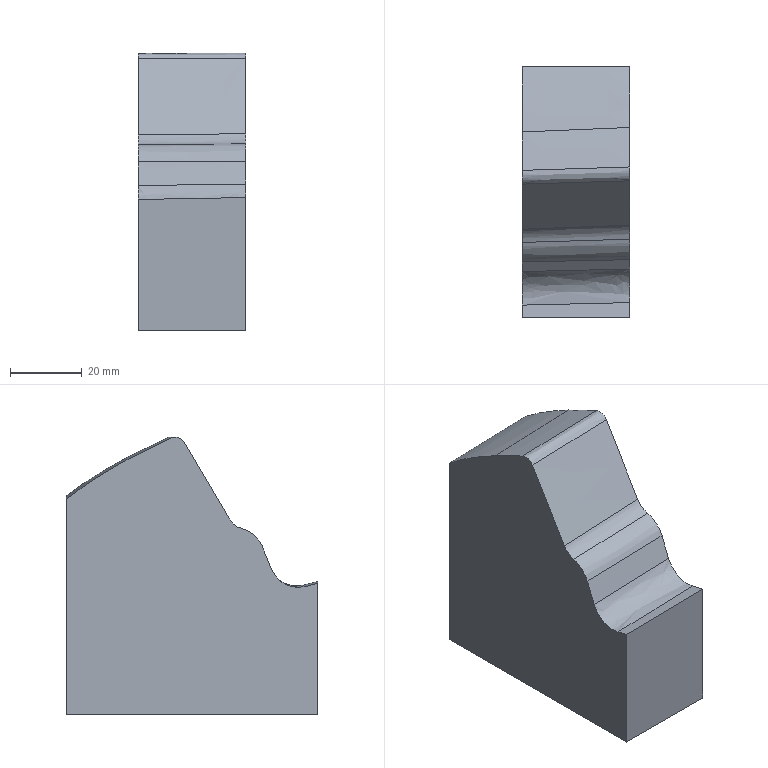Part | NX | features solid 2 | 1 solid | 14 faces | box 30 x 70 x 77.441 mm | volume 125300 mm3 | spline 9 | plane 5
STEP:
#1=CARTESIAN_POINT('',(275.839,786.479,-120.));
#2=VERTEX_POINT('',#1);
#3=CARTESIAN_POINT('',(245.839,786.479,-120.));
#4=VERTEX_POINT('',#3);
#5=CARTESIAN_POINT('',(275.839,786.479,-120.));
#6=DIRECTION('',(1.,0.,0.));
#7=VECTOR('',#6,1000.);
#8=LINE('',#5,#7);
#9=EDGE_CURVE('',#2,#4,#8,.F.);
#10=ORIENTED_EDGE('',*,*,#9,.F.);
#11=CARTESIAN_POINT('',(275.839,716.479,-120.));
#12=VERTEX_POINT('',#11);
#13=CARTESIAN_POINT('',(275.839,776.479,-120.));
#14=DIRECTION('',(0.,-1.,0.));
#15=VECTOR('',#14,1000.);
#16=LINE('',#13,#15);
#17=EDGE_CURVE('',#12,#2,#16,.F.);
#18=ORIENTED_EDGE('',*,*,#17,.F.);
#19=CARTESIAN_POINT('',(245.839,716.479,-120.));
#20=VERTEX_POINT('',#19);
#21=CARTESIAN_POINT('',(275.839,716.479,-120.));
#22=DIRECTION('',(1.,0.,0.));
#23=VECTOR('',#22,1000.);
#24=LINE('',#21,#23);
#25=EDGE_CURVE('',#12,#20,#24,.F.);
#26=ORIENTED_EDGE('',*,*,#25,.T.);
#27=CARTESIAN_POINT('',(245.839,776.479,-120.));
#28=DIRECTION('',(0.,-1.,0.));
#29=VECTOR('',#28,1000.);
#30=LINE('',#27,#29);
#31=EDGE_CURVE('',#20,#4,#30,.F.);
#32=ORIENTED_EDGE('',*,*,#31,.T.);
#33=EDGE_LOOP('',(#10,#18,#26,#32));
#34=FACE_BOUND('',#33,.T.);
#35=CARTESIAN_POINT('',(275.839,776.479,-120.));
#36=DIRECTION('',(0.,0.,1.));
#37=DIRECTION('',(0.,-1.,0.));
#38=AXIS2_PLACEMENT_3D('',#35,#36,#37);
#39=PLANE('',#38);
#40=ADVANCED_FACE('',(#34),#39,.F.);
#41=CARTESIAN_POINT('',(245.839,786.479,-59.905));
#42=VERTEX_POINT('',#41);
#43=CARTESIAN_POINT('',(245.839,768.143,-48.166));
#44=VERTEX_POINT('',#43);
#45=CARTESIAN_POINT('',(245.839,786.479,-59.905));
#46=CARTESIAN_POINT('',(245.839,780.808,-55.303));
#47=CARTESIAN_POINT('',(245.839,774.58,-51.571));
#48=CARTESIAN_POINT('',(245.839,768.143,-48.166));
#49=B_SPLINE_CURVE_WITH_KNOTS('',3,(#45,#46,#47,#48),.UNSPECIFIED.,.F.,.F.,(4,4),(0.,0.02177),.UNSPECIFIED.);
#50=EDGE_CURVE('',#42,#44,#49,.T.);
#51=ORIENTED_EDGE('',*,*,#50,.F.);
#52=CARTESIAN_POINT('',(245.839,786.479,-60.));
#53=DIRECTION('',(0.,0.,-1.));
#54=VECTOR('',#53,1000.);
#55=LINE('',#52,#54);
#56=EDGE_CURVE('',#42,#4,#55,.T.);
#57=ORIENTED_EDGE('',*,*,#56,.T.);
#58=ORIENTED_EDGE('',*,*,#31,.F.);
#59=CARTESIAN_POINT('',(245.839,716.479,-83.363));
#60=VERTEX_POINT('',#59);
#61=CARTESIAN_POINT('',(245.839,716.479,-60.));
#62=DIRECTION('',(0.,0.,-1.));
#63=VECTOR('',#62,1000.);
#64=LINE('',#61,#63);
#65=EDGE_CURVE('',#60,#20,#64,.T.);
#66=ORIENTED_EDGE('',*,*,#65,.F.);
#67=CARTESIAN_POINT('',(245.839,719.964,-84.227));
#68=VERTEX_POINT('',#67);
#69=CARTESIAN_POINT('',(245.839,716.479,-83.363));
#70=CARTESIAN_POINT('',(245.839,717.64,-83.65));
#71=CARTESIAN_POINT('',(245.839,718.801,-83.938));
#72=CARTESIAN_POINT('',(245.839,719.962,-84.226));
#73=B_SPLINE_CURVE_WITH_KNOTS('',3,(#69,#70,#71,#72),.UNSPECIFIED.,.F.,.F.,(4,4),(0.,0.003589),.UNSPECIFIED.);
#74=EDGE_CURVE('',#60,#68,#73,.T.);
#75=ORIENTED_EDGE('',*,*,#74,.T.);
#76=CARTESIAN_POINT('',(245.839,729.312,-79.471));
#77=VERTEX_POINT('',#76);
#78=CARTESIAN_POINT('',(245.839,719.965,-84.227));
#79=CARTESIAN_POINT('',(245.839,721.832,-84.691));
#80=CARTESIAN_POINT('',(245.839,725.84,-84.214));
#81=CARTESIAN_POINT('',(245.839,728.588,-81.253));
#82=CARTESIAN_POINT('',(245.839,729.312,-79.471));
#83=B_SPLINE_CURVE_WITH_KNOTS('',3,(#78,#79,#80,#81,#82),.UNSPECIFIED.,.F.,.F.,(4,1,4),(0.,0.005687,0.01137),.UNSPECIFIED.);
#84=EDGE_CURVE('',#68,#77,#83,.T.);
#85=ORIENTED_EDGE('',*,*,#84,.T.);
#86=CARTESIAN_POINT('',(245.839,731.981,-72.901));
#87=VERTEX_POINT('',#86);
#88=CARTESIAN_POINT('',(245.839,729.312,-79.472));
#89=CARTESIAN_POINT('',(245.839,730.201,-77.282));
#90=CARTESIAN_POINT('',(245.839,731.091,-75.092));
#91=CARTESIAN_POINT('',(245.839,731.98,-72.902));
#92=B_SPLINE_CURVE_WITH_KNOTS('',3,(#88,#89,#90,#91),.UNSPECIFIED.,.F.,.F.,(4,4),(0.00003288,0.007123),.UNSPECIFIED.);
#93=EDGE_CURVE('',#77,#87,#92,.T.);
#94=ORIENTED_EDGE('',*,*,#93,.T.);
#95=CARTESIAN_POINT('',(245.839,737.4,-68.162));
#96=VERTEX_POINT('',#95);
#97=CARTESIAN_POINT('',(245.839,731.981,-72.9));
#98=CARTESIAN_POINT('',(245.839,732.926,-70.575));
#99=CARTESIAN_POINT('',(245.839,734.971,-68.787));
#100=CARTESIAN_POINT('',(245.839,737.401,-68.162));
#101=B_SPLINE_CURVE_WITH_KNOTS('',3,(#97,#98,#99,#100),.UNSPECIFIED.,.F.,.F.,(4,4),(0.,0.007469),.UNSPECIFIED.);
#102=EDGE_CURVE('',#87,#96,#101,.T.);
#103=ORIENTED_EDGE('',*,*,#102,.T.);
#104=CARTESIAN_POINT('',(245.839,741.078,-65.393));
#105=VERTEX_POINT('',#104);
#106=CARTESIAN_POINT('',(245.839,737.4,-68.162));
#107=CARTESIAN_POINT('',(245.839,738.935,-67.766));
#108=CARTESIAN_POINT('',(245.839,740.274,-66.759));
#109=CARTESIAN_POINT('',(245.839,741.078,-65.393));
#110=B_SPLINE_CURVE_WITH_KNOTS('',3,(#106,#107,#108,#109),.UNSPECIFIED.,.F.,.F.,(4,4),(0.,0.004726),.UNSPECIFIED.);
#111=EDGE_CURVE('',#96,#105,#110,.T.);
#112=ORIENTED_EDGE('',*,*,#111,.T.);
#113=CARTESIAN_POINT('',(245.839,753.598,-44.132));
#114=VERTEX_POINT('',#113);
#115=CARTESIAN_POINT('',(245.839,741.078,-65.394));
#116=CARTESIAN_POINT('',(245.839,745.251,-58.307));
#117=CARTESIAN_POINT('',(245.839,749.425,-51.219));
#118=CARTESIAN_POINT('',(245.839,753.598,-44.132));
#119=B_SPLINE_CURVE_WITH_KNOTS('',3,(#115,#116,#117,#118),.UNSPECIFIED.,.F.,.F.,(4,4),(0.000195,0.02487),.UNSPECIFIED.);
#120=EDGE_CURVE('',#105,#114,#119,.T.);
#121=ORIENTED_EDGE('',*,*,#120,.T.);
#122=CARTESIAN_POINT('',(245.839,757.433,-42.927));
#123=VERTEX_POINT('',#122);
#124=CARTESIAN_POINT('',(245.839,753.598,-44.132));
#125=CARTESIAN_POINT('',(245.839,753.974,-43.495));
#126=CARTESIAN_POINT('',(245.839,755.203,-42.538));
#127=CARTESIAN_POINT('',(245.839,756.759,-42.623));
#128=CARTESIAN_POINT('',(245.839,757.433,-42.927));
#129=B_SPLINE_CURVE_WITH_KNOTS('',3,(#124,#125,#126,#127,#128),.UNSPECIFIED.,.F.,.F.,(4,1,4),(0.,0.002188,0.004376),.UNSPECIFIED.);
#130=EDGE_CURVE('',#114,#123,#129,.T.);
#131=ORIENTED_EDGE('',*,*,#130,.T.);
#132=CARTESIAN_POINT('',(245.839,768.143,-48.166));
#133=CARTESIAN_POINT('',(245.839,764.629,-46.307));
#134=CARTESIAN_POINT('',(245.839,761.057,-44.561));
#135=CARTESIAN_POINT('',(245.839,757.433,-42.927));
#136=B_SPLINE_CURVE_WITH_KNOTS('',3,(#132,#133,#134,#135),.UNSPECIFIED.,.F.,.F.,(4,4),(0.002124,0.01405),.UNSPECIFIED.);
#137=EDGE_CURVE('',#44,#123,#136,.T.);
#138=ORIENTED_EDGE('',*,*,#137,.F.);
#139=EDGE_LOOP('',(#51,#57,#58,#66,#75,#85,#94,#103,#112,#121,#131,#138));
#140=FACE_BOUND('',#139,.T.);
#141=CARTESIAN_POINT('',(245.839,726.479,-60.));
#142=DIRECTION('',(-1.,0.,0.));
#143=DIRECTION('',(0.,-1.,0.));
#144=AXIS2_PLACEMENT_3D('',#141,#142,#143);
#145=PLANE('',#144);
#146=ADVANCED_FACE('',(#140),#145,.T.);
#147=CARTESIAN_POINT('',(275.839,716.479,-82.838));
#148=VERTEX_POINT('',#147);
#149=CARTESIAN_POINT('',(275.839,716.479,-60.));
#150=DIRECTION('',(0.,0.,-1.));
#151=VECTOR('',#150,1000.);
#152=LINE('',#149,#151);
#153=EDGE_CURVE('',#148,#12,#152,.T.);
#154=ORIENTED_EDGE('',*,*,#153,.F.);
#155=CARTESIAN_POINT('',(275.839,716.479,-82.838));
#156=CARTESIAN_POINT('',(265.839,716.479,-83.013));
#157=CARTESIAN_POINT('',(255.839,716.479,-83.188));
#158=CARTESIAN_POINT('',(245.839,716.479,-83.363));
#159=B_SPLINE_CURVE_WITH_KNOTS('',3,(#155,#156,#157,#158),.UNSPECIFIED.,.F.,.F.,(4,4),(0.,0.03),.UNSPECIFIED.);
#160=EDGE_CURVE('',#148,#60,#159,.T.);
#161=ORIENTED_EDGE('',*,*,#160,.T.);
#162=ORIENTED_EDGE('',*,*,#65,.T.);
#163=ORIENTED_EDGE('',*,*,#25,.F.);
#164=EDGE_LOOP('',(#154,#161,#162,#163));
#165=FACE_BOUND('',#164,.T.);
#166=CARTESIAN_POINT('',(275.839,716.479,-60.));
#167=DIRECTION('',(0.,-1.,0.));
#168=DIRECTION('',(1.,0.,0.));
#169=AXIS2_PLACEMENT_3D('',#166,#167,#168);
#170=PLANE('',#169);
#171=ADVANCED_FACE('',(#165),#170,.T.);
#172=CARTESIAN_POINT('',(275.839,786.479,-58.959));
#173=VERTEX_POINT('',#172);
#174=CARTESIAN_POINT('',(275.839,786.479,-60.));
#175=DIRECTION('',(0.,0.,-1.));
#176=VECTOR('',#175,1000.);
#177=LINE('',#174,#176);
#178=EDGE_CURVE('',#173,#2,#177,.T.);
#179=ORIENTED_EDGE('',*,*,#178,.F.);
#180=CARTESIAN_POINT('',(275.839,769.372,-48.194));
#181=VERTEX_POINT('',#180);
#182=CARTESIAN_POINT('',(275.839,786.479,-58.959));
#183=CARTESIAN_POINT('',(275.839,781.136,-54.8));
#184=CARTESIAN_POINT('',(275.839,775.346,-51.354));
#185=CARTESIAN_POINT('',(275.839,769.374,-48.195));
#186=B_SPLINE_CURVE_WITH_KNOTS('',3,(#182,#183,#184,#185),.UNSPECIFIED.,.F.,.F.,(4,4),(0.,0.02021),.UNSPECIFIED.);
#187=EDGE_CURVE('',#173,#181,#186,.T.);
#188=ORIENTED_EDGE('',*,*,#187,.T.);
#189=CARTESIAN_POINT('',(275.839,758.369,-42.827));
#190=VERTEX_POINT('',#189);
#191=CARTESIAN_POINT('',(275.839,769.371,-48.193));
#192=CARTESIAN_POINT('',(275.839,765.763,-46.285));
#193=CARTESIAN_POINT('',(275.839,762.092,-44.496));
#194=CARTESIAN_POINT('',(275.839,758.368,-42.826));
#195=B_SPLINE_CURVE_WITH_KNOTS('',3,(#191,#192,#193,#194),.UNSPECIFIED.,.F.,.F.,(4,4),(0.001603,0.01385),.UNSPECIFIED.);
#196=EDGE_CURVE('',#181,#190,#195,.T.);
#197=ORIENTED_EDGE('',*,*,#196,.T.);
#198=CARTESIAN_POINT('',(275.839,754.512,-44.025));
#199=VERTEX_POINT('',#198);
#200=CARTESIAN_POINT('',(275.839,754.512,-44.025));
#201=CARTESIAN_POINT('',(275.839,755.263,-42.743));
#202=CARTESIAN_POINT('',(275.839,757.014,-42.219));
#203=CARTESIAN_POINT('',(275.839,758.37,-42.827));
#204=B_SPLINE_CURVE_WITH_KNOTS('',3,(#200,#201,#202,#203),.UNSPECIFIED.,.F.,.F.,(4,4),(0.,0.004395),.UNSPECIFIED.);
#205=EDGE_CURVE('',#199,#190,#204,.T.);
#206=ORIENTED_EDGE('',*,*,#205,.F.);
#207=CARTESIAN_POINT('',(275.839,742.202,-65.047));
#208=VERTEX_POINT('',#207);
#209=CARTESIAN_POINT('',(275.839,742.203,-65.046));
#210=CARTESIAN_POINT('',(275.839,746.307,-58.039));
#211=CARTESIAN_POINT('',(275.839,750.41,-51.032));
#212=CARTESIAN_POINT('',(275.839,754.512,-44.025));
#213=B_SPLINE_CURVE_WITH_KNOTS('',3,(#209,#210,#211,#212),.UNSPECIFIED.,.F.,.F.,(4,4),(0.0005091,0.02487),.UNSPECIFIED.);
#214=EDGE_CURVE('',#208,#199,#213,.T.);
#215=ORIENTED_EDGE('',*,*,#214,.F.);
#216=CARTESIAN_POINT('',(275.839,738.294,-67.882));
#217=VERTEX_POINT('',#216);
#218=CARTESIAN_POINT('',(275.839,738.307,-67.879));
#219=CARTESIAN_POINT('',(275.839,739.931,-67.523));
#220=CARTESIAN_POINT('',(275.839,741.362,-66.483));
#221=CARTESIAN_POINT('',(275.839,742.202,-65.048));
#222=B_SPLINE_CURVE_WITH_KNOTS('',3,(#218,#219,#220,#221),.UNSPECIFIED.,.F.,.F.,(4,4),(0.,0.004958),.UNSPECIFIED.);
#223=EDGE_CURVE('',#217,#208,#222,.T.);
#224=ORIENTED_EDGE('',*,*,#223,.F.);
#225=CARTESIAN_POINT('',(275.839,732.598,-72.709));
#226=VERTEX_POINT('',#225);
#227=CARTESIAN_POINT('',(275.839,732.601,-72.701));
#228=CARTESIAN_POINT('',(275.839,733.576,-70.285));
#229=CARTESIAN_POINT('',(275.839,735.748,-68.447));
#230=CARTESIAN_POINT('',(275.839,738.29,-67.883));
#231=B_SPLINE_CURVE_WITH_KNOTS('',3,(#227,#228,#229,#230),.UNSPECIFIED.,.F.,.F.,(4,4),(0.,0.007755),.UNSPECIFIED.);
#232=EDGE_CURVE('',#226,#217,#231,.T.);
#233=ORIENTED_EDGE('',*,*,#232,.F.);
#234=CARTESIAN_POINT('',(275.839,730.018,-79.103));
#235=VERTEX_POINT('',#234);
#236=CARTESIAN_POINT('',(275.839,730.018,-79.103));
#237=CARTESIAN_POINT('',(275.839,730.878,-76.973));
#238=CARTESIAN_POINT('',(275.839,731.737,-74.842));
#239=CARTESIAN_POINT('',(275.839,732.597,-72.712));
#240=B_SPLINE_CURVE_WITH_KNOTS('',3,(#236,#237,#238,#239),.UNSPECIFIED.,.F.,.F.,(4,4),(0.00002376,0.006916),.UNSPECIFIED.);
#241=EDGE_CURVE('',#235,#226,#240,.T.);
#242=ORIENTED_EDGE('',*,*,#241,.F.);
#243=CARTESIAN_POINT('',(275.839,720.661,-83.875));
#244=VERTEX_POINT('',#243);
#245=CARTESIAN_POINT('',(275.839,720.665,-83.876));
#246=CARTESIAN_POINT('',(275.839,722.534,-84.341));
#247=CARTESIAN_POINT('',(275.839,726.55,-83.861));
#248=CARTESIAN_POINT('',(275.839,729.298,-80.89));
#249=CARTESIAN_POINT('',(275.839,730.018,-79.103));
#250=B_SPLINE_CURVE_WITH_KNOTS('',3,(#245,#246,#247,#248,#249),.UNSPECIFIED.,.F.,.F.,(4,1,4),(0.,0.005697,0.01139),.UNSPECIFIED.);
#251=EDGE_CURVE('',#244,#235,#250,.T.);
#252=ORIENTED_EDGE('',*,*,#251,.F.);
#253=CARTESIAN_POINT('',(275.839,716.479,-82.838));
#254=CARTESIAN_POINT('',(275.839,717.873,-83.183));
#255=CARTESIAN_POINT('',(275.839,719.266,-83.528));
#256=CARTESIAN_POINT('',(275.839,720.66,-83.875));
#257=B_SPLINE_CURVE_WITH_KNOTS('',3,(#253,#254,#255,#256),.UNSPECIFIED.,.F.,.F.,(4,4),(0.,0.004308),.UNSPECIFIED.);
#258=EDGE_CURVE('',#148,#244,#257,.T.);
#259=ORIENTED_EDGE('',*,*,#258,.F.);
#260=ORIENTED_EDGE('',*,*,#153,.T.);
#261=ORIENTED_EDGE('',*,*,#17,.T.);
#262=EDGE_LOOP('',(#179,#188,#197,#206,#215,#224,#233,#242,#252,#259,#260,#261));
#263=FACE_BOUND('',#262,.T.);
#264=CARTESIAN_POINT('',(275.839,726.479,-60.));
#265=DIRECTION('',(-1.,0.,0.));
#266=DIRECTION('',(0.,-1.,0.));
#267=AXIS2_PLACEMENT_3D('',#264,#265,#266);
#268=PLANE('',#267);
#269=ADVANCED_FACE('',(#263),#268,.F.);
#270=ORIENTED_EDGE('',*,*,#56,.F.);
#271=CARTESIAN_POINT('',(245.839,786.479,-59.905));
#272=CARTESIAN_POINT('',(255.839,786.479,-59.575));
#273=CARTESIAN_POINT('',(265.839,786.479,-59.26));
#274=CARTESIAN_POINT('',(275.839,786.479,-58.959));
#275=B_SPLINE_CURVE_WITH_KNOTS('',3,(#271,#272,#273,#274),.UNSPECIFIED.,.F.,.F.,(4,4),(0.,0.03001),.UNSPECIFIED.);
#276=EDGE_CURVE('',#42,#173,#275,.T.);
#277=ORIENTED_EDGE('',*,*,#276,.T.);
#278=ORIENTED_EDGE('',*,*,#178,.T.);
#279=ORIENTED_EDGE('',*,*,#9,.T.);
#280=EDGE_LOOP('',(#270,#277,#278,#279));
#281=FACE_BOUND('',#280,.T.);
#282=CARTESIAN_POINT('',(275.839,786.479,-60.));
#283=DIRECTION('',(0.,-1.,0.));
#284=DIRECTION('',(1.,0.,0.));
#285=AXIS2_PLACEMENT_3D('',#282,#283,#284);
#286=PLANE('',#285);
#287=ADVANCED_FACE('',(#281),#286,.F.);
#288=ORIENTED_EDGE('',*,*,#276,.F.);
#289=ORIENTED_EDGE('',*,*,#50,.T.);
#290=CARTESIAN_POINT('',(275.839,769.374,-48.195));
#291=CARTESIAN_POINT('',(265.838,768.982,-48.191));
#292=CARTESIAN_POINT('',(255.838,768.573,-48.182));
#293=CARTESIAN_POINT('',(245.839,768.143,-48.166));
#294=B_SPLINE_CURVE_WITH_KNOTS('',3,(#290,#291,#292,#293),.UNSPECIFIED.,.F.,.F.,(4,4),(0.79,0.9686),.UNSPECIFIED.);
#295=EDGE_CURVE('',#181,#44,#294,.T.);
#296=ORIENTED_EDGE('',*,*,#295,.F.);
#297=ORIENTED_EDGE('',*,*,#187,.F.);
#298=EDGE_LOOP('',(#288,#289,#296,#297));
#299=FACE_BOUND('',#298,.T.);
#300=CARTESIAN_POINT('',(276.02,769.382,-48.195));
#301=CARTESIAN_POINT('',(276.026,773.342,-50.29));
#302=CARTESIAN_POINT('',(276.033,777.232,-52.501));
#303=CARTESIAN_POINT('',(276.043,780.983,-54.841));
#304=CARTESIAN_POINT('',(276.04,784.525,-57.337));
#305=CARTESIAN_POINT('',(276.008,787.811,-60.014));
#306=CARTESIAN_POINT('',(269.947,769.144,-48.193));
#307=CARTESIAN_POINT('',(269.952,773.104,-50.288));
#308=CARTESIAN_POINT('',(269.959,776.994,-52.499));
#309=CARTESIAN_POINT('',(269.967,780.745,-54.839));
#310=CARTESIAN_POINT('',(269.963,784.287,-57.335));
#311=CARTESIAN_POINT('',(269.93,787.573,-60.012));
#312=CARTESIAN_POINT('',(263.875,768.9,-48.189));
#313=CARTESIAN_POINT('',(263.878,772.86,-50.284));
#314=CARTESIAN_POINT('',(263.884,776.751,-52.495));
#315=CARTESIAN_POINT('',(263.891,780.502,-54.835));
#316=CARTESIAN_POINT('',(263.886,784.044,-57.331));
#317=CARTESIAN_POINT('',(263.851,787.33,-60.009));
#318=CARTESIAN_POINT('',(257.802,768.651,-48.183));
#319=CARTESIAN_POINT('',(257.804,772.612,-50.278));
#320=CARTESIAN_POINT('',(257.809,776.502,-52.49));
#321=CARTESIAN_POINT('',(257.815,780.253,-54.829));
#322=CARTESIAN_POINT('',(257.808,783.796,-57.325));
#323=CARTESIAN_POINT('',(257.772,787.082,-60.003));
#324=CARTESIAN_POINT('',(251.73,768.397,-48.176));
#325=CARTESIAN_POINT('',(251.73,772.357,-50.271));
#326=CARTESIAN_POINT('',(251.733,776.248,-52.482));
#327=CARTESIAN_POINT('',(251.738,779.998,-54.821));
#328=CARTESIAN_POINT('',(251.73,783.541,-57.317));
#329=CARTESIAN_POINT('',(251.692,786.827,-59.995));
#330=CARTESIAN_POINT('',(245.658,768.135,-48.166));
#331=CARTESIAN_POINT('',(245.657,772.096,-50.261));
#332=CARTESIAN_POINT('',(245.658,775.987,-52.472));
#333=CARTESIAN_POINT('',(245.661,779.738,-54.811));
#334=CARTESIAN_POINT('',(245.651,783.281,-57.307));
#335=CARTESIAN_POINT('',(245.611,786.567,-59.985));
#336=B_SPLINE_SURFACE_WITH_KNOTS('',5,5,((#300,#301,#302,#303,#304,#305),(#306,#307,#308,#309,#310,#311),(#312,#313,#314,#315,#316,#317),(#318,#319,#320,#321,#322,#323),(#324,#325,#326,#327,#328,#329),(#330,#331,#332,#333,#334,#335)),.UNSPECIFIED.,.F.,.F.,.F.,(6,6),(6,6),(0.8526,0.9789),(0.,0.2902),.PIECEWISE_BEZIER_KNOTS.);
#337=ADVANCED_FACE('',(#299),#336,.F.);
#338=ORIENTED_EDGE('',*,*,#295,.T.);
#339=ORIENTED_EDGE('',*,*,#137,.T.);
#340=CARTESIAN_POINT('',(275.839,758.368,-42.826));
#341=CARTESIAN_POINT('',(265.09,758.062,-42.872));
#342=CARTESIAN_POINT('',(255.09,757.75,-42.906));
#343=CARTESIAN_POINT('',(245.839,757.433,-42.927));
#344=B_SPLINE_CURVE_WITH_KNOTS('',3,(#340,#341,#342,#343),.UNSPECIFIED.,.F.,.F.,(4,4),(0.5417,0.9262),.UNSPECIFIED.);
#345=EDGE_CURVE('',#190,#123,#344,.T.);
#346=ORIENTED_EDGE('',*,*,#345,.F.);
#347=ORIENTED_EDGE('',*,*,#196,.F.);
#348=EDGE_LOOP('',(#338,#339,#346,#347));
#349=FACE_BOUND('',#348,.T.);
#350=CARTESIAN_POINT('',(276.079,757.983,-42.65));
#351=CARTESIAN_POINT('',(276.044,763.838,-45.259));
#352=CARTESIAN_POINT('',(276.019,769.442,-48.227));
#353=CARTESIAN_POINT('',(269.994,757.86,-42.698));
#354=CARTESIAN_POINT('',(269.962,763.701,-45.307));
#355=CARTESIAN_POINT('',(269.941,769.292,-48.272));
#356=CARTESIAN_POINT('',(263.909,757.736,-42.747));
#357=CARTESIAN_POINT('',(263.881,763.564,-45.355));
#358=CARTESIAN_POINT('',(263.863,769.141,-48.317));
#359=CARTESIAN_POINT('',(257.825,757.612,-42.797));
#360=CARTESIAN_POINT('',(257.8,763.425,-45.404));
#361=CARTESIAN_POINT('',(257.786,768.989,-48.362));
#362=CARTESIAN_POINT('',(251.742,757.487,-42.847));
#363=CARTESIAN_POINT('',(251.721,763.285,-45.453));
#364=CARTESIAN_POINT('',(251.71,768.835,-48.408));
#365=CARTESIAN_POINT('',(245.659,757.36,-42.898));
#366=CARTESIAN_POINT('',(245.641,763.144,-45.503));
#367=CARTESIAN_POINT('',(245.634,768.679,-48.455));
#368=B_SPLINE_SURFACE_WITH_KNOTS('',5,2,((#350,#351,#352),(#353,#354,#355),(#356,#357,#358),(#359,#360,#361),(#362,#363,#364),(#365,#366,#367)),.UNSPECIFIED.,.F.,.F.,.F.,(6,6),(3,3),(0.7902,0.97),(0.006349,0.8931),.PIECEWISE_BEZIER_KNOTS.);
#369=ADVANCED_FACE('',(#349),#368,.F.);
#370=ORIENTED_EDGE('',*,*,#205,.T.);
#371=ORIENTED_EDGE('',*,*,#345,.T.);
#372=ORIENTED_EDGE('',*,*,#130,.F.);
#373=CARTESIAN_POINT('',(275.839,754.512,-44.025));
#374=CARTESIAN_POINT('',(265.837,754.225,-44.064));
#375=CARTESIAN_POINT('',(255.837,753.92,-44.099));
#376=CARTESIAN_POINT('',(245.839,753.598,-44.132));
#377=B_SPLINE_CURVE_WITH_KNOTS('',3,(#373,#374,#375,#376),.UNSPECIFIED.,.F.,.F.,(4,4),(0.79,0.969),.UNSPECIFIED.);
#378=EDGE_CURVE('',#114,#199,#377,.F.);
#379=ORIENTED_EDGE('',*,*,#378,.T.);
#380=EDGE_LOOP('',(#370,#371,#372,#379));
#381=FACE_BOUND('',#380,.T.);
#382=CARTESIAN_POINT('',(276.025,758.375,-42.826));
#383=CARTESIAN_POINT('',(276.015,756.977,-42.2));
#384=CARTESIAN_POINT('',(276.012,755.291,-42.703));
#385=CARTESIAN_POINT('',(276.078,754.519,-44.024));
#386=CARTESIAN_POINT('',(269.94,758.202,-42.852));
#387=CARTESIAN_POINT('',(269.931,756.804,-42.225));
#388=CARTESIAN_POINT('',(269.933,755.118,-42.727));
#389=CARTESIAN_POINT('',(269.993,754.345,-44.048));
#390=CARTESIAN_POINT('',(263.855,758.021,-42.876));
#391=CARTESIAN_POINT('',(263.849,756.624,-42.248));
#392=CARTESIAN_POINT('',(263.855,754.938,-42.75));
#393=CARTESIAN_POINT('',(263.909,754.165,-44.071));
#394=CARTESIAN_POINT('',(257.77,757.832,-42.897));
#395=CARTESIAN_POINT('',(257.766,756.435,-42.268));
#396=CARTESIAN_POINT('',(257.777,754.754,-42.771));
#397=CARTESIAN_POINT('',(257.825,753.979,-44.092));
#398=CARTESIAN_POINT('',(251.686,757.634,-42.914));
#399=CARTESIAN_POINT('',(251.684,756.237,-42.285));
#400=CARTESIAN_POINT('',(251.7,754.563,-42.792));
#401=CARTESIAN_POINT('',(251.741,753.788,-44.113));
#402=CARTESIAN_POINT('',(245.601,757.425,-42.928));
#403=CARTESIAN_POINT('',(245.603,756.028,-42.298));
#404=CARTESIAN_POINT('',(245.624,754.369,-42.813));
#405=CARTESIAN_POINT('',(245.659,753.592,-44.133));
#406=B_SPLINE_SURFACE_WITH_KNOTS('',5,3,((#382,#383,#384,#385),(#386,#387,#388,#389),(#390,#391,#392,#393),(#394,#395,#396,#397),(#398,#399,#400,#401),(#402,#403,#404,#405)),.UNSPECIFIED.,.F.,.F.,.F.,(6,6),(4,4),(0.7886,0.9701),(0.,1.),.PIECEWISE_BEZIER_KNOTS.);
#407=ADVANCED_FACE('',(#381),#406,.T.);
#408=ORIENTED_EDGE('',*,*,#214,.T.);
#409=ORIENTED_EDGE('',*,*,#378,.F.);
#410=ORIENTED_EDGE('',*,*,#120,.F.);
#411=CARTESIAN_POINT('',(245.839,741.078,-65.394));
#412=CARTESIAN_POINT('',(248.329,741.175,-65.366));
#413=CARTESIAN_POINT('',(253.353,741.369,-65.311));
#414=CARTESIAN_POINT('',(259.74,741.611,-65.238));
#415=CARTESIAN_POINT('',(264.894,741.804,-65.177));
#416=CARTESIAN_POINT('',(268.163,741.925,-65.138));
#417=CARTESIAN_POINT('',(270.41,742.007,-65.111));
#418=CARTESIAN_POINT('',(271.778,742.057,-65.094));
#419=CARTESIAN_POINT('',(272.845,742.096,-65.081));
#420=CARTESIAN_POINT('',(274.176,742.144,-65.065));
#421=CARTESIAN_POINT('',(275.281,742.183,-65.052));
#422=CARTESIAN_POINT('',(275.839,742.203,-65.046));
#423=B_SPLINE_CURVE_WITH_KNOTS('',3,(#411,#412,#413,#414,#415,#416,#417,#418,#419,#420,#421,#422),.UNSPECIFIED.,.F.,.F.,(4,1,1,1,1,1,1,1,1,4),(0.07845,0.2022,0.3259,0.3878,0.4497,0.4806,0.4961,0.5116,0.5425,0.5734),.UNSPECIFIED.);
#424=EDGE_CURVE('',#105,#208,#423,.T.);
#425=ORIENTED_EDGE('',*,*,#424,.T.);
#426=EDGE_LOOP('',(#408,#409,#410,#425));
#427=FACE_BOUND('',#426,.T.);
#428=CARTESIAN_POINT('',(276.027,754.518,-44.024));
#429=CARTESIAN_POINT('',(276.044,753.778,-45.289));
#430=CARTESIAN_POINT('',(276.062,753.038,-46.554));
#431=CARTESIAN_POINT('',(276.08,752.298,-47.819));
#432=CARTESIAN_POINT('',(276.11,751.053,-49.947));
#433=CARTESIAN_POINT('',(276.14,749.807,-52.074));
#434=CARTESIAN_POINT('',(276.153,749.302,-52.937));
#435=CARTESIAN_POINT('',(276.174,748.417,-54.45));
#436=CARTESIAN_POINT('',(276.196,747.532,-55.963));
#437=CARTESIAN_POINT('',(276.205,747.152,-56.612));
#438=CARTESIAN_POINT('',(276.235,745.891,-58.768));
#439=CARTESIAN_POINT('',(276.266,744.629,-60.924));
#440=CARTESIAN_POINT('',(276.287,743.748,-62.43));
#441=CARTESIAN_POINT('',(276.308,742.866,-63.937));
#442=CARTESIAN_POINT('',(276.33,741.985,-65.443));
#443=CARTESIAN_POINT('',(269.698,754.336,-44.049));
#444=CARTESIAN_POINT('',(269.718,753.596,-45.313));
#445=CARTESIAN_POINT('',(269.738,752.855,-46.578));
#446=CARTESIAN_POINT('',(269.758,752.114,-47.842));
#447=CARTESIAN_POINT('',(269.791,750.868,-49.969));
#448=CARTESIAN_POINT('',(269.824,749.622,-52.097));
#449=CARTESIAN_POINT('',(269.838,749.117,-52.959));
#450=CARTESIAN_POINT('',(269.861,748.231,-54.471));
#451=CARTESIAN_POINT('',(269.885,747.345,-55.984));
#452=CARTESIAN_POINT('',(269.895,746.965,-56.633));
#453=CARTESIAN_POINT('',(269.929,745.702,-58.788));
#454=CARTESIAN_POINT('',(269.963,744.44,-60.943));
#455=CARTESIAN_POINT('',(269.986,743.558,-62.449));
#456=CARTESIAN_POINT('',(270.01,742.675,-63.955));
#457=CARTESIAN_POINT('',(270.033,741.793,-65.461));
#458=CARTESIAN_POINT('',(263.439,754.151,-44.072));
#459=CARTESIAN_POINT('',(263.461,753.41,-45.336));
#460=CARTESIAN_POINT('',(263.482,752.668,-46.6));
#461=CARTESIAN_POINT('',(263.504,751.927,-47.864));
#462=CARTESIAN_POINT('',(263.54,750.68,-49.991));
#463=CARTESIAN_POINT('',(263.577,749.433,-52.117));
#464=CARTESIAN_POINT('',(263.592,748.927,-52.98));
#465=CARTESIAN_POINT('',(263.618,748.041,-54.491));
#466=CARTESIAN_POINT('',(263.643,747.154,-56.003));
#467=CARTESIAN_POINT('',(263.655,746.773,-56.652));
#468=CARTESIAN_POINT('',(263.692,745.51,-58.807));
#469=CARTESIAN_POINT('',(263.728,744.246,-60.961));
#470=CARTESIAN_POINT('',(263.754,743.363,-62.467));
#471=CARTESIAN_POINT('',(263.78,742.481,-63.972));
#472=CARTESIAN_POINT('',(263.806,741.598,-65.478));
#473=CARTESIAN_POINT('',(257.262,753.962,-44.094));
#474=CARTESIAN_POINT('',(257.285,753.22,-45.357));
#475=CARTESIAN_POINT('',(257.309,752.478,-46.621));
#476=CARTESIAN_POINT('',(257.332,751.736,-47.885));
#477=CARTESIAN_POINT('',(257.372,750.488,-50.01));
#478=CARTESIAN_POINT('',(257.411,749.24,-52.136));
#479=CARTESIAN_POINT('',(257.427,748.734,-52.999));
#480=CARTESIAN_POINT('',(257.456,747.847,-54.51));
#481=CARTESIAN_POINT('',(257.484,746.96,-56.021));
#482=CARTESIAN_POINT('',(257.496,746.579,-56.67));
#483=CARTESIAN_POINT('',(257.536,745.314,-58.824));
#484=CARTESIAN_POINT('',(257.576,744.05,-60.978));
#485=CARTESIAN_POINT('',(257.604,743.166,-62.483));
#486=CARTESIAN_POINT('',(257.632,742.283,-63.988));
#487=CARTESIAN_POINT('',(257.66,741.399,-65.493));
#488=CARTESIAN_POINT('',(251.18,753.77,-44.114));
#489=CARTESIAN_POINT('',(251.205,753.028,-45.377));
#490=CARTESIAN_POINT('',(251.23,752.285,-46.641));
#491=CARTESIAN_POINT('',(251.256,751.543,-47.904));
#492=CARTESIAN_POINT('',(251.298,750.294,-50.029));
#493=CARTESIAN_POINT('',(251.341,749.045,-52.155));
#494=CARTESIAN_POINT('',(251.358,748.538,-53.017));
#495=CARTESIAN_POINT('',(251.389,747.651,-54.527));
#496=CARTESIAN_POINT('',(251.419,746.763,-56.038));
#497=CARTESIAN_POINT('',(251.432,746.382,-56.687));
#498=CARTESIAN_POINT('',(251.475,745.116,-58.84));
#499=CARTESIAN_POINT('',(251.518,743.851,-60.994));
#500=CARTESIAN_POINT('',(251.549,742.967,-62.498));
#501=CARTESIAN_POINT('',(251.579,742.082,-64.003));
#502=CARTESIAN_POINT('',(251.609,741.198,-65.508));
#503=CARTESIAN_POINT('',(245.206,753.578,-44.134));
#504=CARTESIAN_POINT('',(245.233,752.835,-45.397));
#505=CARTESIAN_POINT('',(245.26,752.092,-46.66));
#506=CARTESIAN_POINT('',(245.287,751.349,-47.923));
#507=CARTESIAN_POINT('',(245.333,750.099,-50.048));
#508=CARTESIAN_POINT('',(245.378,748.849,-52.173));
#509=CARTESIAN_POINT('',(245.397,748.342,-53.034));
#510=CARTESIAN_POINT('',(245.429,747.454,-54.545));
#511=CARTESIAN_POINT('',(245.462,746.565,-56.055));
#512=CARTESIAN_POINT('',(245.476,746.184,-56.703));
#513=CARTESIAN_POINT('',(245.522,744.918,-58.856));
#514=CARTESIAN_POINT('',(245.568,743.651,-61.009));
#515=CARTESIAN_POINT('',(245.601,742.766,-62.513));
#516=CARTESIAN_POINT('',(245.633,741.881,-64.017));
#517=CARTESIAN_POINT('',(245.666,740.997,-65.522));
#518=B_SPLINE_SURFACE_WITH_KNOTS('',5,5,((#428,#429,#430,#431,#432,#433,#434,#435,#436,#437,#438,#439,#440,#441,#442),(#443,#444,#445,#446,#447,#448,#449,#450,#451,#452,#453,#454,#455,#456,#457),(#458,#459,#460,#461,#462,#463,#464,#465,#466,#467,#468,#469,#470,#471,#472),(#473,#474,#475,#476,#477,#478,#479,#480,#481,#482,#483,#484,#485,#486,#487),(#488,#489,#490,#491,#492,#493,#494,#495,#496,#497,#498,#499,#500,#501,#502),(#503,#504,#505,#506,#507,#508,#509,#510,#511,#512,#513,#514,#515,#516,#517)),.UNSPECIFIED.,.F.,.F.,.F.,(6,6),(6,3,3,3,6),(0.7831,0.9712),(0.,0.2947,0.4958,0.6471,0.9981),.UNSPECIFIED.);
#519=ADVANCED_FACE('',(#427),#518,.T.);
#520=ORIENTED_EDGE('',*,*,#223,.T.);
#521=ORIENTED_EDGE('',*,*,#424,.F.);
#522=ORIENTED_EDGE('',*,*,#111,.F.);
#523=CARTESIAN_POINT('',(275.839,738.307,-67.879));
#524=CARTESIAN_POINT('',(265.792,738.023,-67.973));
#525=CARTESIAN_POINT('',(255.809,737.722,-68.071));
#526=CARTESIAN_POINT('',(245.839,737.4,-68.162));
#527=B_SPLINE_CURVE_WITH_KNOTS('',3,(#523,#524,#525,#526),.UNSPECIFIED.,.F.,.F.,(4,4),(0.4407,0.9258),.UNSPECIFIED.);
#528=EDGE_CURVE('',#217,#96,#527,.T.);
#529=ORIENTED_EDGE('',*,*,#528,.F.);
#530=EDGE_LOOP('',(#520,#521,#522,#529));
#531=FACE_BOUND('',#530,.T.);
#532=CARTESIAN_POINT('',(245.486,741.064,-65.397));
#533=CARTESIAN_POINT('',(245.514,740.586,-66.211));
#534=CARTESIAN_POINT('',(245.546,739.948,-66.93));
#535=CARTESIAN_POINT('',(245.582,739.174,-67.513));
#536=CARTESIAN_POINT('',(245.621,738.307,-67.928));
#537=CARTESIAN_POINT('',(245.659,737.394,-68.163));
#538=CARTESIAN_POINT('',(247.887,741.158,-65.37));
#539=CARTESIAN_POINT('',(247.914,740.678,-66.187));
#540=CARTESIAN_POINT('',(247.947,740.037,-66.909));
#541=CARTESIAN_POINT('',(247.984,739.26,-67.493));
#542=CARTESIAN_POINT('',(248.022,738.389,-67.908));
#543=CARTESIAN_POINT('',(248.06,737.472,-68.142));
#544=CARTESIAN_POINT('',(250.291,741.251,-65.343));
#545=CARTESIAN_POINT('',(250.318,740.77,-66.163));
#546=CARTESIAN_POINT('',(250.351,740.126,-66.887));
#547=CARTESIAN_POINT('',(250.388,739.345,-67.472));
#548=CARTESIAN_POINT('',(250.426,738.47,-67.887));
#549=CARTESIAN_POINT('',(250.464,737.548,-68.119));
#550=CARTESIAN_POINT('',(252.696,741.344,-65.315));
#551=CARTESIAN_POINT('',(252.724,740.861,-66.138));
#552=CARTESIAN_POINT('',(252.757,740.215,-66.865));
#553=CARTESIAN_POINT('',(252.793,739.43,-67.452));
#554=CARTESIAN_POINT('',(252.831,738.55,-67.867));
#555=CARTESIAN_POINT('',(252.869,737.624,-68.097));
#556=CARTESIAN_POINT('',(256.388,741.486,-65.273));
#557=CARTESIAN_POINT('',(256.416,741.,-66.101));
#558=CARTESIAN_POINT('',(256.449,740.349,-66.831));
#559=CARTESIAN_POINT('',(256.485,739.558,-67.42));
#560=CARTESIAN_POINT('',(256.524,738.671,-67.834));
#561=CARTESIAN_POINT('',(256.561,737.739,-68.062));
#562=CARTESIAN_POINT('',(260.082,741.626,-65.23));
#563=CARTESIAN_POINT('',(260.11,741.137,-66.063));
#564=CARTESIAN_POINT('',(260.142,740.481,-66.797));
#565=CARTESIAN_POINT('',(260.179,739.684,-67.388));
#566=CARTESIAN_POINT('',(260.217,738.79,-67.802));
#567=CARTESIAN_POINT('',(260.255,737.851,-68.027));
#568=CARTESIAN_POINT('',(261.369,741.674,-65.215));
#569=CARTESIAN_POINT('',(261.397,741.185,-66.05));
#570=CARTESIAN_POINT('',(261.429,740.527,-66.786));
#571=CARTESIAN_POINT('',(261.466,739.727,-67.377));
#572=CARTESIAN_POINT('',(261.504,738.831,-67.791));
#573=CARTESIAN_POINT('',(261.542,737.89,-68.015));
#574=CARTESIAN_POINT('',(265.065,741.812,-65.172));
#575=CARTESIAN_POINT('',(265.093,741.32,-66.012));
#576=CARTESIAN_POINT('',(265.125,740.658,-66.752));
#577=CARTESIAN_POINT('',(265.162,739.852,-67.345));
#578=CARTESIAN_POINT('',(265.199,738.949,-67.759));
#579=CARTESIAN_POINT('',(265.237,738.001,-67.979));
#580=CARTESIAN_POINT('',(268.766,741.949,-65.129));
#581=CARTESIAN_POINT('',(268.793,741.454,-65.974));
#582=CARTESIAN_POINT('',(268.826,740.786,-66.718));
#583=CARTESIAN_POINT('',(268.862,739.974,-67.314));
#584=CARTESIAN_POINT('',(268.9,739.064,-67.726));
#585=CARTESIAN_POINT('',(268.937,738.109,-67.944));
#586=CARTESIAN_POINT('',(271.181,742.036,-65.101));
#587=CARTESIAN_POINT('',(271.208,741.54,-65.949));
#588=CARTESIAN_POINT('',(271.24,740.869,-66.696));
#589=CARTESIAN_POINT('',(271.276,740.053,-67.293));
#590=CARTESIAN_POINT('',(271.314,739.138,-67.705));
#591=CARTESIAN_POINT('',(271.351,738.179,-67.921));
#592=CARTESIAN_POINT('',(273.599,742.123,-65.073));
#593=CARTESIAN_POINT('',(273.626,741.625,-65.925));
#594=CARTESIAN_POINT('',(273.658,740.951,-66.674));
#595=CARTESIAN_POINT('',(273.694,740.131,-67.273));
#596=CARTESIAN_POINT('',(273.731,739.212,-67.685));
#597=CARTESIAN_POINT('',(273.768,738.248,-67.898));
#598=CARTESIAN_POINT('',(276.021,742.209,-65.046));
#599=CARTESIAN_POINT('',(276.048,741.709,-65.901));
#600=CARTESIAN_POINT('',(276.08,741.032,-66.653));
#601=CARTESIAN_POINT('',(276.115,740.208,-67.252));
#602=CARTESIAN_POINT('',(276.152,739.284,-67.664));
#603=CARTESIAN_POINT('',(276.188,738.317,-67.876));
#604=B_SPLINE_SURFACE_WITH_KNOTS('',5,5,((#532,#533,#534,#535,#536,#537),(#538,#539,#540,#541,#542,#543),(#544,#545,#546,#547,#548,#549),(#550,#551,#552,#553,#554,#555),(#556,#557,#558,#559,#560,#561),(#562,#563,#564,#565,#566,#567),(#568,#569,#570,#571,#572,#573),(#574,#575,#576,#577,#578,#579),(#580,#581,#582,#583,#584,#585),(#586,#587,#588,#589,#590,#591),(#592,#593,#594,#595,#596,#597),(#598,#599,#600,#601,#602,#603)),.UNSPECIFIED.,.F.,.F.,.F.,(6,3,3,6),(6,6),(0.07127,0.266,0.3702,0.5649),(0.,1.),.UNSPECIFIED.);
#605=ADVANCED_FACE('',(#531),#604,.F.);
#606=ORIENTED_EDGE('',*,*,#232,.T.);
#607=ORIENTED_EDGE('',*,*,#528,.T.);
#608=ORIENTED_EDGE('',*,*,#102,.F.);
#609=CARTESIAN_POINT('',(245.839,731.981,-72.9));
#610=CARTESIAN_POINT('',(255.939,732.217,-72.837));
#611=CARTESIAN_POINT('',(265.875,732.414,-72.769));
#612=CARTESIAN_POINT('',(275.839,732.601,-72.701));
#613=B_SPLINE_CURVE_WITH_KNOTS('',3,(#609,#610,#611,#612),.UNSPECIFIED.,.F.,.F.,(4,4),(0.07006,0.5549),.UNSPECIFIED.);
#614=EDGE_CURVE('',#87,#226,#613,.T.);
#615=ORIENTED_EDGE('',*,*,#614,.T.);
#616=EDGE_LOOP('',(#606,#607,#608,#615));
#617=FACE_BOUND('',#616,.T.);
#618=CARTESIAN_POINT('',(276.019,738.339,-67.872));
#619=CARTESIAN_POINT('',(276.05,736.814,-68.2));
#620=CARTESIAN_POINT('',(276.082,735.37,-68.901));
#621=CARTESIAN_POINT('',(276.114,734.127,-69.948));
#622=CARTESIAN_POINT('',(276.141,733.191,-71.252));
#623=CARTESIAN_POINT('',(276.163,732.607,-72.699));
#624=CARTESIAN_POINT('',(272.689,738.278,-67.896));
#625=CARTESIAN_POINT('',(272.721,736.753,-68.224));
#626=CARTESIAN_POINT('',(272.754,735.308,-68.924));
#627=CARTESIAN_POINT('',(272.785,734.065,-69.971));
#628=CARTESIAN_POINT('',(272.813,733.129,-71.275));
#629=CARTESIAN_POINT('',(272.835,732.545,-72.721));
#630=CARTESIAN_POINT('',(269.363,738.216,-67.92));
#631=CARTESIAN_POINT('',(269.395,736.691,-68.248));
#632=CARTESIAN_POINT('',(269.429,735.246,-68.947));
#633=CARTESIAN_POINT('',(269.461,734.002,-69.994));
#634=CARTESIAN_POINT('',(269.489,733.066,-71.298));
#635=CARTESIAN_POINT('',(269.511,732.482,-72.744));
#636=CARTESIAN_POINT('',(266.038,738.152,-67.944));
#637=CARTESIAN_POINT('',(266.071,736.627,-68.271));
#638=CARTESIAN_POINT('',(266.105,735.182,-68.971));
#639=CARTESIAN_POINT('',(266.137,733.938,-70.016));
#640=CARTESIAN_POINT('',(266.165,733.001,-71.32));
#641=CARTESIAN_POINT('',(266.188,732.417,-72.767));
#642=CARTESIAN_POINT('',(259.961,738.033,-67.987));
#643=CARTESIAN_POINT('',(259.995,736.508,-68.314));
#644=CARTESIAN_POINT('',(260.03,735.062,-69.013));
#645=CARTESIAN_POINT('',(260.063,733.818,-70.058));
#646=CARTESIAN_POINT('',(260.092,732.881,-71.361));
#647=CARTESIAN_POINT('',(260.115,732.295,-72.807));
#648=CARTESIAN_POINT('',(253.845,737.905,-68.03));
#649=CARTESIAN_POINT('',(253.881,736.38,-68.356));
#650=CARTESIAN_POINT('',(253.917,734.935,-69.054));
#651=CARTESIAN_POINT('',(253.952,733.69,-70.099));
#652=CARTESIAN_POINT('',(253.982,732.752,-71.402));
#653=CARTESIAN_POINT('',(254.005,732.166,-72.848));
#654=CARTESIAN_POINT('',(251.067,737.846,-68.049));
#655=CARTESIAN_POINT('',(251.104,736.321,-68.375));
#656=CARTESIAN_POINT('',(251.141,734.875,-69.073));
#657=CARTESIAN_POINT('',(251.176,733.63,-70.117));
#658=CARTESIAN_POINT('',(251.206,732.691,-71.42));
#659=CARTESIAN_POINT('',(251.23,732.105,-72.866));
#660=CARTESIAN_POINT('',(248.28,737.784,-68.068));
#661=CARTESIAN_POINT('',(248.318,736.259,-68.394));
#662=CARTESIAN_POINT('',(248.356,734.813,-69.091));
#663=CARTESIAN_POINT('',(248.392,733.567,-70.135));
#664=CARTESIAN_POINT('',(248.422,732.629,-71.438));
#665=CARTESIAN_POINT('',(248.446,732.042,-72.883));
#666=CARTESIAN_POINT('',(245.488,737.72,-68.087));
#667=CARTESIAN_POINT('',(245.526,736.194,-68.412));
#668=CARTESIAN_POINT('',(245.565,734.748,-69.109));
#669=CARTESIAN_POINT('',(245.602,733.503,-70.153));
#670=CARTESIAN_POINT('',(245.633,732.564,-71.455));
#671=CARTESIAN_POINT('',(245.656,731.977,-72.901));
#672=B_SPLINE_SURFACE_WITH_KNOTS('',5,5,((#618,#619,#620,#621,#622,#623),(#624,#625,#626,#627,#628,#629),(#630,#631,#632,#633,#634,#635),(#636,#637,#638,#639,#640,#641),(#642,#643,#644,#645,#646,#647),(#648,#649,#650,#651,#652,#653),(#654,#655,#656,#657,#658,#659),(#660,#661,#662,#663,#664,#665),(#666,#667,#668,#669,#670,#671)),.UNSPECIFIED.,.F.,.F.,.F.,(6,3,6),(6,6),(0.4399,0.7098,0.9329),(0.0272,1.),.UNSPECIFIED.);
#673=ADVANCED_FACE('',(#617),#672,.T.);
#674=ORIENTED_EDGE('',*,*,#241,.T.);
#675=ORIENTED_EDGE('',*,*,#614,.F.);
#676=ORIENTED_EDGE('',*,*,#93,.F.);
#677=CARTESIAN_POINT('',(245.839,729.312,-79.472));
#678=CARTESIAN_POINT('',(255.816,729.573,-79.356));
#679=CARTESIAN_POINT('',(265.795,729.8,-79.231));
#680=CARTESIAN_POINT('',(275.839,730.018,-79.103));
#681=B_SPLINE_CURVE_WITH_KNOTS('',3,(#677,#678,#679,#680),.UNSPECIFIED.,.F.,.F.,(4,4),(0.5062,0.6431),.UNSPECIFIED.);
#682=EDGE_CURVE('',#77,#235,#681,.T.);
#683=ORIENTED_EDGE('',*,*,#682,.T.);
#684=EDGE_LOOP('',(#674,#675,#676,#683));
#685=FACE_BOUND('',#684,.T.);
#686=CARTESIAN_POINT('',(245.659,729.295,-79.504));
#687=CARTESIAN_POINT('',(245.614,730.193,-77.292));
#688=CARTESIAN_POINT('',(245.568,731.09,-75.079));
#689=CARTESIAN_POINT('',(245.523,731.988,-72.867));
#690=CARTESIAN_POINT('',(246.25,729.31,-79.497));
#691=CARTESIAN_POINT('',(246.205,730.208,-77.285));
#692=CARTESIAN_POINT('',(246.159,731.106,-75.072));
#693=CARTESIAN_POINT('',(246.114,732.003,-72.86));
#694=CARTESIAN_POINT('',(246.841,729.326,-79.49));
#695=CARTESIAN_POINT('',(246.795,730.223,-77.277));
#696=CARTESIAN_POINT('',(246.75,731.121,-75.065));
#697=CARTESIAN_POINT('',(246.704,732.019,-72.852));
#698=CARTESIAN_POINT('',(247.432,729.341,-79.483));
#699=CARTESIAN_POINT('',(247.386,730.239,-77.27));
#700=CARTESIAN_POINT('',(247.341,731.136,-75.058));
#701=CARTESIAN_POINT('',(247.295,732.034,-72.845));
#702=CARTESIAN_POINT('',(253.515,729.498,-79.41));
#703=CARTESIAN_POINT('',(253.47,730.395,-77.197));
#704=CARTESIAN_POINT('',(253.425,731.291,-74.984));
#705=CARTESIAN_POINT('',(253.38,732.188,-72.771));
#706=CARTESIAN_POINT('',(259.597,729.645,-79.334));
#707=CARTESIAN_POINT('',(259.553,730.541,-77.121));
#708=CARTESIAN_POINT('',(259.508,731.436,-74.908));
#709=CARTESIAN_POINT('',(259.464,732.332,-72.694));
#710=CARTESIAN_POINT('',(265.099,729.772,-79.265));
#711=CARTESIAN_POINT('',(265.055,730.667,-77.051));
#712=CARTESIAN_POINT('',(265.011,731.561,-74.837));
#713=CARTESIAN_POINT('',(264.966,732.456,-72.623));
#714=CARTESIAN_POINT('',(270.618,729.895,-79.193));
#715=CARTESIAN_POINT('',(270.574,730.789,-76.979));
#716=CARTESIAN_POINT('',(270.53,731.683,-74.765));
#717=CARTESIAN_POINT('',(270.486,732.576,-72.551));
#718=CARTESIAN_POINT('',(276.148,730.016,-79.122));
#719=CARTESIAN_POINT('',(276.104,730.909,-76.907));
#720=CARTESIAN_POINT('',(276.06,731.801,-74.692));
#721=CARTESIAN_POINT('',(276.016,732.694,-72.478));
#722=B_SPLINE_SURFACE_WITH_KNOTS('',5,3,((#686,#687,#688,#689),(#690,#691,#692,#693),(#694,#695,#696,#697),(#698,#699,#700,#701),(#702,#703,#704,#705),(#706,#707,#708,#709),(#710,#711,#712,#713),(#714,#715,#716,#717),(#718,#719,#720,#721)),.UNSPECIFIED.,.F.,.F.,.F.,(6,3,6),(4,4),(0.5008,0.5142,0.6387),(0.,0.973),.UNSPECIFIED.);
#723=ADVANCED_FACE('',(#685),#722,.T.);
#724=ORIENTED_EDGE('',*,*,#251,.T.);
#725=ORIENTED_EDGE('',*,*,#682,.F.);
#726=ORIENTED_EDGE('',*,*,#84,.F.);
#727=CARTESIAN_POINT('',(275.839,720.665,-83.876));
#728=CARTESIAN_POINT('',(265.811,720.449,-83.998));
#729=CARTESIAN_POINT('',(255.833,720.225,-84.117));
#730=CARTESIAN_POINT('',(245.839,719.965,-84.227));
#731=B_SPLINE_CURVE_WITH_KNOTS('',3,(#727,#728,#729,#730),.UNSPECIFIED.,.F.,.F.,(4,4),(0.3164,0.4624),.UNSPECIFIED.);
#732=EDGE_CURVE('',#68,#244,#731,.F.);
#733=ORIENTED_EDGE('',*,*,#732,.T.);
#734=EDGE_LOOP('',(#724,#725,#726,#733));
#735=FACE_BOUND('',#734,.T.);
#736=CARTESIAN_POINT('',(245.658,719.961,-84.229));
#737=CARTESIAN_POINT('',(245.632,721.07,-84.505));
#738=CARTESIAN_POINT('',(245.602,722.228,-84.583));
#739=CARTESIAN_POINT('',(245.571,723.388,-84.451));
#740=CARTESIAN_POINT('',(245.506,725.61,-83.778));
#741=CARTESIAN_POINT('',(245.442,727.461,-82.378));
#742=CARTESIAN_POINT('',(245.412,728.251,-81.518));
#743=CARTESIAN_POINT('',(245.385,728.87,-80.536));
#744=CARTESIAN_POINT('',(245.362,729.299,-79.477));
#745=CARTESIAN_POINT('',(250.247,720.08,-84.178));
#746=CARTESIAN_POINT('',(250.223,721.189,-84.454));
#747=CARTESIAN_POINT('',(250.195,722.348,-84.532));
#748=CARTESIAN_POINT('',(250.164,723.508,-84.4));
#749=CARTESIAN_POINT('',(250.101,725.73,-83.727));
#750=CARTESIAN_POINT('',(250.039,727.582,-82.326));
#751=CARTESIAN_POINT('',(250.01,728.372,-81.465));
#752=CARTESIAN_POINT('',(249.983,728.991,-80.483));
#753=CARTESIAN_POINT('',(249.96,729.42,-79.424));
#754=CARTESIAN_POINT('',(254.835,720.193,-84.126));
#755=CARTESIAN_POINT('',(254.811,721.303,-84.402));
#756=CARTESIAN_POINT('',(254.784,722.461,-84.48));
#757=CARTESIAN_POINT('',(254.755,723.622,-84.348));
#758=CARTESIAN_POINT('',(254.694,725.845,-83.674));
#759=CARTESIAN_POINT('',(254.633,727.697,-82.273));
#760=CARTESIAN_POINT('',(254.604,728.487,-81.412));
#761=CARTESIAN_POINT('',(254.578,729.105,-80.429));
#762=CARTESIAN_POINT('',(254.555,729.535,-79.369));
#763=CARTESIAN_POINT('',(259.421,720.301,-84.073));
#764=CARTESIAN_POINT('',(259.398,721.411,-84.349));
#765=CARTESIAN_POINT('',(259.372,722.57,-84.427));
#766=CARTESIAN_POINT('',(259.343,723.731,-84.294));
#767=CARTESIAN_POINT('',(259.284,725.955,-83.62));
#768=CARTESIAN_POINT('',(259.224,727.807,-82.218));
#769=CARTESIAN_POINT('',(259.196,728.597,-81.356));
#770=CARTESIAN_POINT('',(259.17,729.215,-80.373));
#771=CARTESIAN_POINT('',(259.147,729.644,-79.313));
#772=CARTESIAN_POINT('',(265.541,720.44,-84.));
#773=CARTESIAN_POINT('',(265.52,721.55,-84.277));
#774=CARTESIAN_POINT('',(265.495,722.71,-84.354));
#775=CARTESIAN_POINT('',(265.467,723.872,-84.222));
#776=CARTESIAN_POINT('',(265.409,726.096,-83.547));
#777=CARTESIAN_POINT('',(265.351,727.948,-82.144));
#778=CARTESIAN_POINT('',(265.323,728.738,-81.282));
#779=CARTESIAN_POINT('',(265.297,729.357,-80.298));
#780=CARTESIAN_POINT('',(265.275,729.785,-79.237));
#781=CARTESIAN_POINT('',(271.674,720.575,-83.926));
#782=CARTESIAN_POINT('',(271.653,721.685,-84.203));
#783=CARTESIAN_POINT('',(271.628,722.845,-84.281));
#784=CARTESIAN_POINT('',(271.601,724.007,-84.148));
#785=CARTESIAN_POINT('',(271.545,726.232,-83.473));
#786=CARTESIAN_POINT('',(271.487,728.085,-82.068));
#787=CARTESIAN_POINT('',(271.46,728.875,-81.205));
#788=CARTESIAN_POINT('',(271.434,729.493,-80.221));
#789=CARTESIAN_POINT('',(271.412,729.921,-79.159));
#790=CARTESIAN_POINT('',(273.208,720.608,-83.908));
#791=CARTESIAN_POINT('',(273.188,721.719,-84.184));
#792=CARTESIAN_POINT('',(273.163,722.879,-84.262));
#793=CARTESIAN_POINT('',(273.137,724.041,-84.129));
#794=CARTESIAN_POINT('',(273.08,726.266,-83.454));
#795=CARTESIAN_POINT('',(273.023,728.119,-82.049));
#796=CARTESIAN_POINT('',(272.995,728.909,-81.186));
#797=CARTESIAN_POINT('',(272.97,729.527,-80.201));
#798=CARTESIAN_POINT('',(272.948,729.955,-79.14));
#799=CARTESIAN_POINT('',(274.744,720.641,-83.889));
#800=CARTESIAN_POINT('',(274.723,721.752,-84.166));
#801=CARTESIAN_POINT('',(274.699,722.912,-84.244));
#802=CARTESIAN_POINT('',(274.672,724.075,-84.111));
#803=CARTESIAN_POINT('',(274.616,726.3,-83.435));
#804=CARTESIAN_POINT('',(274.559,728.153,-82.03));
#805=CARTESIAN_POINT('',(274.532,728.943,-81.167));
#806=CARTESIAN_POINT('',(274.506,729.561,-80.182));
#807=CARTESIAN_POINT('',(274.484,729.989,-79.12));
#808=CARTESIAN_POINT('',(276.28,720.674,-83.871));
#809=CARTESIAN_POINT('',(276.26,721.785,-84.147));
#810=CARTESIAN_POINT('',(276.236,722.945,-84.225));
#811=CARTESIAN_POINT('',(276.209,724.108,-84.092));
#812=CARTESIAN_POINT('',(276.153,726.333,-83.416));
#813=CARTESIAN_POINT('',(276.096,728.186,-82.011));
#814=CARTESIAN_POINT('',(276.069,728.976,-81.148));
#815=CARTESIAN_POINT('',(276.043,729.594,-80.163));
#816=CARTESIAN_POINT('',(276.021,730.022,-79.101));
#817=B_SPLINE_SURFACE_WITH_KNOTS('',5,5,((#736,#737,#738,#739,#740,#741,#742,#743,#744),(#745,#746,#747,#748,#749,#750,#751,#752,#753),(#754,#755,#756,#757,#758,#759,#760,#761,#762),(#763,#764,#765,#766,#767,#768,#769,#770,#771),(#772,#773,#774,#775,#776,#777,#778,#779,#780),(#781,#782,#783,#784,#785,#786,#787,#788,#789),(#790,#791,#792,#793,#794,#795,#796,#797,#798),(#799,#800,#801,#802,#803,#804,#805,#806,#807),(#808,#809,#810,#811,#812,#813,#814,#815,#816)),.UNSPECIFIED.,.F.,.F.,.F.,(6,3,6),(6,3,6),(0.5367,0.6484,0.6857),(0.,0.5,1.),.UNSPECIFIED.);
#818=ADVANCED_FACE('',(#735),#817,.T.);
#819=ORIENTED_EDGE('',*,*,#258,.T.);
#820=ORIENTED_EDGE('',*,*,#732,.F.);
#821=ORIENTED_EDGE('',*,*,#74,.F.);
#822=ORIENTED_EDGE('',*,*,#160,.F.);
#823=EDGE_LOOP('',(#819,#820,#821,#822));
#824=FACE_BOUND('',#823,.T.);
#825=CARTESIAN_POINT('',(276.019,716.454,-82.828));
#826=CARTESIAN_POINT('',(245.644,716.454,-83.36));
#827=CARTESIAN_POINT('',(276.025,717.864,-83.177));
#828=CARTESIAN_POINT('',(245.65,717.864,-83.709));
#829=CARTESIAN_POINT('',(276.031,719.275,-83.527));
#830=CARTESIAN_POINT('',(245.656,719.275,-84.058));
#831=CARTESIAN_POINT('',(276.037,720.685,-83.877));
#832=CARTESIAN_POINT('',(245.662,720.685,-84.409));
#833=(BOUNDED_SURFACE()B_SPLINE_SURFACE(3,1,((#825,#826),(#827,#828),(#829,#830),(#831,#832)),.CYLINDRICAL_SURF.,.F.,.F.,.F.)B_SPLINE_SURFACE_WITH_KNOTS((4,4),(2,2),(0.9712,0.9875),(0.1435,0.1848),.PIECEWISE_BEZIER_KNOTS.)GEOMETRIC_REPRESENTATION_ITEM()RATIONAL_B_SPLINE_SURFACE(((1.,1.),(1.,1.),(1.,1.),(1.,1.)))REPRESENTATION_ITEM('')SURFACE());
#834=ADVANCED_FACE('',(#824),#833,.T.);
#835=CLOSED_SHELL('',(#40,#146,#171,#269,#287,#337,#369,#407,#519,#605,#673,#723,#818,#834));
#836=MANIFOLD_SOLID_BREP('',#835);
#837=(LENGTH_UNIT()NAMED_UNIT(*)SI_UNIT(.MILLI.,.METRE.));
#838=UNCERTAINTY_MEASURE_WITH_UNIT(LENGTH_MEASURE(0.07711),#837,'','');
#839=(NAMED_UNIT(*)PLANE_ANGLE_UNIT()SI_UNIT($,.RADIAN.));
#840=(NAMED_UNIT(*)SI_UNIT($,.STERADIAN.)SOLID_ANGLE_UNIT());
#841=(GEOMETRIC_REPRESENTATION_CONTEXT(3)GLOBAL_UNCERTAINTY_ASSIGNED_CONTEXT((#838))GLOBAL_UNIT_ASSIGNED_CONTEXT((#837,#839,#840))REPRESENTATION_CONTEXT('',''));
#842=ADVANCED_BREP_SHAPE_REPRESENTATION('',(#836),#841);